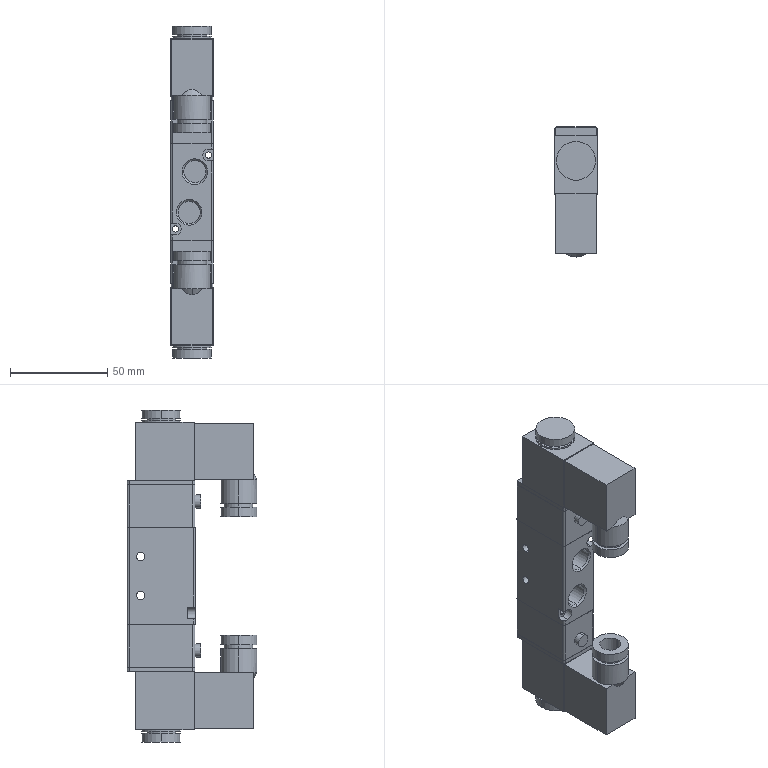Part | NX | features BREP 1 | 1 solid | 166 faces | box 22 x 66.8 x 170.8 mm | volume 156847 mm3 | plane 79 | cylinder 74 | cone 13 | commonest cylinder face diameters 2 x22 15 x8 18.6 x8 20 x8 11.445 x6 3.2 x4